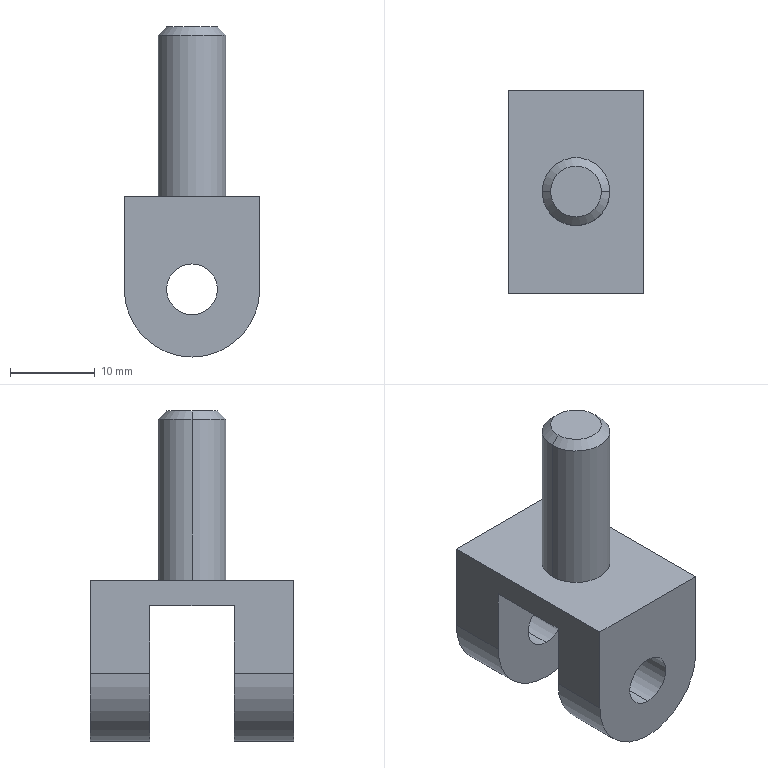Part | SolidWorks | features ICE 3, Chamfer 1, Extrusion 1 | 1 solid | 21 faces | box 16 x 24 x 39 mm | volume 4949 mm3 | cylinder 10 | plane 9 | cone 2 | commonest cylinder face diameters 6 x4 16 x4 8 x2
STEP:
#1=CARTESIAN_POINT('',(3.,0.,31.));
#2=VERTEX_POINT('',#1);
#3=CARTESIAN_POINT('',(-3.,0.,31.));
#4=VERTEX_POINT('',#3);
#5=CARTESIAN_POINT('',(0.,0.,31.));
#6=DIRECTION('',(0.,0.,1.));
#7=DIRECTION('',(1.,0.,0.));
#8=AXIS2_PLACEMENT_3D('',#5,#6,#7);
#9=CIRCLE('',#8,3.);
#10=EDGE_CURVE('',#2,#4,#9,.T.);
#11=ORIENTED_EDGE('',*,*,#10,.F.);
#12=CARTESIAN_POINT('',(4.,0.,30.));
#13=VERTEX_POINT('',#12);
#14=CARTESIAN_POINT('',(3.,0.,31.));
#15=DIRECTION('',(0.7071,0.,-0.7071));
#16=VECTOR('',#15,1000.);
#17=LINE('',#14,#16);
#18=EDGE_CURVE('',#2,#13,#17,.T.);
#19=ORIENTED_EDGE('',*,*,#18,.T.);
#20=CARTESIAN_POINT('',(-4.,0.,30.));
#21=VERTEX_POINT('',#20);
#22=CARTESIAN_POINT('',(0.,0.,30.));
#23=DIRECTION('',(0.,0.,-1.));
#24=DIRECTION('',(1.,0.,0.));
#25=AXIS2_PLACEMENT_3D('',#22,#23,#24);
#26=CIRCLE('',#25,4.);
#27=EDGE_CURVE('',#21,#13,#26,.T.);
#28=ORIENTED_EDGE('',*,*,#27,.F.);
#29=CARTESIAN_POINT('',(-3.,0.,31.));
#30=DIRECTION('',(-0.7071,0.,-0.7071));
#31=VECTOR('',#30,1000.);
#32=LINE('',#29,#31);
#33=EDGE_CURVE('',#4,#21,#32,.T.);
#34=ORIENTED_EDGE('',*,*,#33,.F.);
#35=EDGE_LOOP('',(#11,#19,#28,#34));
#36=FACE_OUTER_BOUND('',#35,.T.);
#37=CARTESIAN_POINT('',(0.,0.,31.));
#38=DIRECTION('',(0.,0.,-1.));
#39=DIRECTION('',(-1.,0.,0.));
#40=AXIS2_PLACEMENT_3D('',#37,#38,#39);
#41=CONICAL_SURFACE('',#40,3.,0.7854);
#42=ADVANCED_FACE('',(#36),#41,.T.);
#43=CARTESIAN_POINT('',(0.,12.,-3.));
#44=VERTEX_POINT('',#43);
#45=CARTESIAN_POINT('',(0.,12.,3.));
#46=VERTEX_POINT('',#45);
#47=CARTESIAN_POINT('',(0.,12.,0.));
#48=DIRECTION('',(0.,1.,0.));
#49=DIRECTION('',(0.,0.,1.));
#50=AXIS2_PLACEMENT_3D('',#47,#48,#49);
#51=CIRCLE('',#50,3.);
#52=EDGE_CURVE('',#44,#46,#51,.T.);
#53=ORIENTED_EDGE('',*,*,#52,.T.);
#54=CARTESIAN_POINT('',(0.,5.,3.));
#55=VERTEX_POINT('',#54);
#56=CARTESIAN_POINT('',(0.,22.,3.));
#57=DIRECTION('',(0.,-1.,0.));
#58=VECTOR('',#57,1000.);
#59=LINE('',#56,#58);
#60=EDGE_CURVE('',#46,#55,#59,.T.);
#61=ORIENTED_EDGE('',*,*,#60,.T.);
#62=CARTESIAN_POINT('',(0.,5.,-3.));
#63=VERTEX_POINT('',#62);
#64=CARTESIAN_POINT('',(0.,5.,0.));
#65=DIRECTION('',(0.,1.,0.));
#66=DIRECTION('',(0.,0.,1.));
#67=AXIS2_PLACEMENT_3D('',#64,#65,#66);
#68=CIRCLE('',#67,3.);
#69=EDGE_CURVE('',#63,#55,#68,.T.);
#70=ORIENTED_EDGE('',*,*,#69,.F.);
#71=CARTESIAN_POINT('',(0.,22.,-3.));
#72=DIRECTION('',(0.,-1.,0.));
#73=VECTOR('',#72,1000.);
#74=LINE('',#71,#73);
#75=EDGE_CURVE('',#44,#63,#74,.T.);
#76=ORIENTED_EDGE('',*,*,#75,.F.);
#77=EDGE_LOOP('',(#53,#61,#70,#76));
#78=FACE_OUTER_BOUND('',#77,.T.);
#79=CARTESIAN_POINT('',(0.,22.,0.));
#80=DIRECTION('',(0.,-1.,0.));
#81=DIRECTION('',(0.,0.,-1.));
#82=AXIS2_PLACEMENT_3D('',#79,#80,#81);
#83=CYLINDRICAL_SURFACE('',#82,3.);
#84=ADVANCED_FACE('',(#78),#83,.F.);
#85=CARTESIAN_POINT('',(0.,-5.,3.));
#86=VERTEX_POINT('',#85);
#87=CARTESIAN_POINT('',(0.,-5.,-3.));
#88=VERTEX_POINT('',#87);
#89=CARTESIAN_POINT('',(0.,-5.,0.));
#90=DIRECTION('',(0.,-1.,0.));
#91=DIRECTION('',(0.,0.,-1.));
#92=AXIS2_PLACEMENT_3D('',#89,#90,#91);
#93=CIRCLE('',#92,3.);
#94=EDGE_CURVE('',#86,#88,#93,.T.);
#95=ORIENTED_EDGE('',*,*,#94,.F.);
#96=CARTESIAN_POINT('',(0.,-12.,3.));
#97=VERTEX_POINT('',#96);
#98=CARTESIAN_POINT('',(0.,22.,3.));
#99=DIRECTION('',(0.,-1.,0.));
#100=VECTOR('',#99,1000.);
#101=LINE('',#98,#100);
#102=EDGE_CURVE('',#86,#97,#101,.T.);
#103=ORIENTED_EDGE('',*,*,#102,.T.);
#104=CARTESIAN_POINT('',(0.,-12.,-3.));
#105=VERTEX_POINT('',#104);
#106=CARTESIAN_POINT('',(0.,-12.,0.));
#107=DIRECTION('',(0.,-1.,0.));
#108=DIRECTION('',(0.,0.,-1.));
#109=AXIS2_PLACEMENT_3D('',#106,#107,#108);
#110=CIRCLE('',#109,3.);
#111=EDGE_CURVE('',#97,#105,#110,.T.);
#112=ORIENTED_EDGE('',*,*,#111,.T.);
#113=CARTESIAN_POINT('',(0.,22.,-3.));
#114=DIRECTION('',(0.,-1.,0.));
#115=VECTOR('',#114,1000.);
#116=LINE('',#113,#115);
#117=EDGE_CURVE('',#88,#105,#116,.T.);
#118=ORIENTED_EDGE('',*,*,#117,.F.);
#119=EDGE_LOOP('',(#95,#103,#112,#118));
#120=FACE_OUTER_BOUND('',#119,.T.);
#121=CARTESIAN_POINT('',(0.,22.,0.));
#122=DIRECTION('',(0.,-1.,0.));
#123=DIRECTION('',(0.,0.,-1.));
#124=AXIS2_PLACEMENT_3D('',#121,#122,#123);
#125=CYLINDRICAL_SURFACE('',#124,3.);
#126=ADVANCED_FACE('',(#120),#125,.F.);
#127=ORIENTED_EDGE('',*,*,#27,.T.);
#128=CARTESIAN_POINT('',(4.,0.,11.));
#129=VERTEX_POINT('',#128);
#130=CARTESIAN_POINT('',(4.,0.,31.));
#131=DIRECTION('',(0.,0.,-1.));
#132=VECTOR('',#131,1000.);
#133=LINE('',#130,#132);
#134=EDGE_CURVE('',#13,#129,#133,.T.);
#135=ORIENTED_EDGE('',*,*,#134,.T.);
#136=CARTESIAN_POINT('',(-4.,0.,11.));
#137=VERTEX_POINT('',#136);
#138=CARTESIAN_POINT('',(0.,0.,11.));
#139=DIRECTION('',(0.,0.,1.));
#140=DIRECTION('',(-1.,0.,0.));
#141=AXIS2_PLACEMENT_3D('',#138,#139,#140);
#142=CIRCLE('',#141,4.);
#143=EDGE_CURVE('',#129,#137,#142,.T.);
#144=ORIENTED_EDGE('',*,*,#143,.T.);
#145=CARTESIAN_POINT('',(-4.,0.,31.));
#146=DIRECTION('',(0.,0.,-1.));
#147=VECTOR('',#146,1000.);
#148=LINE('',#145,#147);
#149=EDGE_CURVE('',#21,#137,#148,.T.);
#150=ORIENTED_EDGE('',*,*,#149,.F.);
#151=EDGE_LOOP('',(#127,#135,#144,#150));
#152=FACE_OUTER_BOUND('',#151,.T.);
#153=CARTESIAN_POINT('',(0.,0.,31.));
#154=DIRECTION('',(0.,0.,-1.));
#155=DIRECTION('',(-1.,0.,0.));
#156=AXIS2_PLACEMENT_3D('',#153,#154,#155);
#157=CYLINDRICAL_SURFACE('',#156,4.);
#158=ADVANCED_FACE('',(#152),#157,.T.);
#159=CARTESIAN_POINT('',(-8.,-5.,0.));
#160=VERTEX_POINT('',#159);
#161=CARTESIAN_POINT('',(0.,-5.,-8.));
#162=VERTEX_POINT('',#161);
#163=CARTESIAN_POINT('',(0.,-5.,0.));
#164=DIRECTION('',(0.,-1.,0.));
#165=DIRECTION('',(0.,0.,-1.));
#166=AXIS2_PLACEMENT_3D('',#163,#164,#165);
#167=CIRCLE('',#166,8.);
#168=EDGE_CURVE('',#160,#162,#167,.T.);
#169=ORIENTED_EDGE('',*,*,#168,.T.);
#170=CARTESIAN_POINT('',(0.,-12.,-8.));
#171=VERTEX_POINT('',#170);
#172=CARTESIAN_POINT('',(0.,12.,-8.));
#173=DIRECTION('',(0.,-1.,0.));
#174=VECTOR('',#173,1000.);
#175=LINE('',#172,#174);
#176=EDGE_CURVE('',#162,#171,#175,.T.);
#177=ORIENTED_EDGE('',*,*,#176,.T.);
#178=CARTESIAN_POINT('',(-8.,-12.,0.));
#179=VERTEX_POINT('',#178);
#180=CARTESIAN_POINT('',(0.,-12.,0.));
#181=DIRECTION('',(0.,1.,0.));
#182=DIRECTION('',(0.,0.,1.));
#183=AXIS2_PLACEMENT_3D('',#180,#181,#182);
#184=CIRCLE('',#183,8.);
#185=EDGE_CURVE('',#171,#179,#184,.T.);
#186=ORIENTED_EDGE('',*,*,#185,.T.);
#187=CARTESIAN_POINT('',(-8.,12.,0.));
#188=DIRECTION('',(0.,-1.,0.));
#189=VECTOR('',#188,1000.);
#190=LINE('',#187,#189);
#191=EDGE_CURVE('',#160,#179,#190,.T.);
#192=ORIENTED_EDGE('',*,*,#191,.F.);
#193=EDGE_LOOP('',(#169,#177,#186,#192));
#194=FACE_OUTER_BOUND('',#193,.T.);
#195=CARTESIAN_POINT('',(0.,12.,0.));
#196=DIRECTION('',(0.,-1.,0.));
#197=DIRECTION('',(0.,0.,-1.));
#198=AXIS2_PLACEMENT_3D('',#195,#196,#197);
#199=CYLINDRICAL_SURFACE('',#198,8.);
#200=ADVANCED_FACE('',(#194),#199,.T.);
#201=CARTESIAN_POINT('',(0.,12.,-8.));
#202=VERTEX_POINT('',#201);
#203=CARTESIAN_POINT('',(-8.,12.,0.));
#204=VERTEX_POINT('',#203);
#205=CARTESIAN_POINT('',(0.,12.,0.));
#206=DIRECTION('',(0.,1.,0.));
#207=DIRECTION('',(0.,0.,1.));
#208=AXIS2_PLACEMENT_3D('',#205,#206,#207);
#209=CIRCLE('',#208,8.);
#210=EDGE_CURVE('',#202,#204,#209,.T.);
#211=ORIENTED_EDGE('',*,*,#210,.F.);
#212=CARTESIAN_POINT('',(0.,5.,-8.));
#213=VERTEX_POINT('',#212);
#214=CARTESIAN_POINT('',(0.,12.,-8.));
#215=DIRECTION('',(0.,-1.,0.));
#216=VECTOR('',#215,1000.);
#217=LINE('',#214,#216);
#218=EDGE_CURVE('',#202,#213,#217,.T.);
#219=ORIENTED_EDGE('',*,*,#218,.T.);
#220=CARTESIAN_POINT('',(-8.,5.,0.));
#221=VERTEX_POINT('',#220);
#222=CARTESIAN_POINT('',(0.,5.,0.));
#223=DIRECTION('',(0.,1.,0.));
#224=DIRECTION('',(0.,0.,1.));
#225=AXIS2_PLACEMENT_3D('',#222,#223,#224);
#226=CIRCLE('',#225,8.);
#227=EDGE_CURVE('',#213,#221,#226,.T.);
#228=ORIENTED_EDGE('',*,*,#227,.T.);
#229=CARTESIAN_POINT('',(-8.,12.,0.));
#230=DIRECTION('',(0.,-1.,0.));
#231=VECTOR('',#230,1000.);
#232=LINE('',#229,#231);
#233=EDGE_CURVE('',#204,#221,#232,.T.);
#234=ORIENTED_EDGE('',*,*,#233,.F.);
#235=EDGE_LOOP('',(#211,#219,#228,#234));
#236=FACE_OUTER_BOUND('',#235,.T.);
#237=CARTESIAN_POINT('',(0.,12.,0.));
#238=DIRECTION('',(0.,-1.,0.));
#239=DIRECTION('',(0.,0.,-1.));
#240=AXIS2_PLACEMENT_3D('',#237,#238,#239);
#241=CYLINDRICAL_SURFACE('',#240,8.);
#242=ADVANCED_FACE('',(#236),#241,.T.);
#243=ORIENTED_EDGE('',*,*,#218,.F.);
#244=CARTESIAN_POINT('',(8.,12.,0.));
#245=VERTEX_POINT('',#244);
#246=CARTESIAN_POINT('',(0.,12.,0.));
#247=DIRECTION('',(0.,1.,0.));
#248=DIRECTION('',(0.,0.,1.));
#249=AXIS2_PLACEMENT_3D('',#246,#247,#248);
#250=CIRCLE('',#249,8.);
#251=EDGE_CURVE('',#245,#202,#250,.T.);
#252=ORIENTED_EDGE('',*,*,#251,.F.);
#253=CARTESIAN_POINT('',(8.,5.,0.));
#254=VERTEX_POINT('',#253);
#255=CARTESIAN_POINT('',(8.,12.,0.));
#256=DIRECTION('',(0.,-1.,0.));
#257=VECTOR('',#256,1000.);
#258=LINE('',#255,#257);
#259=EDGE_CURVE('',#245,#254,#258,.T.);
#260=ORIENTED_EDGE('',*,*,#259,.T.);
#261=CARTESIAN_POINT('',(0.,5.,0.));
#262=DIRECTION('',(0.,1.,0.));
#263=DIRECTION('',(0.,0.,1.));
#264=AXIS2_PLACEMENT_3D('',#261,#262,#263);
#265=CIRCLE('',#264,8.);
#266=EDGE_CURVE('',#254,#213,#265,.T.);
#267=ORIENTED_EDGE('',*,*,#266,.T.);
#268=EDGE_LOOP('',(#243,#252,#260,#267));
#269=FACE_OUTER_BOUND('',#268,.T.);
#270=CARTESIAN_POINT('',(0.,12.,0.));
#271=DIRECTION('',(0.,-1.,0.));
#272=DIRECTION('',(0.,0.,-1.));
#273=AXIS2_PLACEMENT_3D('',#270,#271,#272);
#274=CYLINDRICAL_SURFACE('',#273,8.);
#275=ADVANCED_FACE('',(#269),#274,.T.);
#276=CARTESIAN_POINT('',(-8.,-12.,11.));
#277=VERTEX_POINT('',#276);
#278=CARTESIAN_POINT('',(8.,-12.,11.));
#279=VERTEX_POINT('',#278);
#280=CARTESIAN_POINT('',(-8.,-12.,11.));
#281=DIRECTION('',(1.,0.,0.));
#282=VECTOR('',#281,1000.);
#283=LINE('',#280,#282);
#284=EDGE_CURVE('',#277,#279,#283,.T.);
#285=ORIENTED_EDGE('',*,*,#284,.T.);
#286=CARTESIAN_POINT('',(8.,12.,11.));
#287=VERTEX_POINT('',#286);
#288=CARTESIAN_POINT('',(8.,12.,11.));
#289=DIRECTION('',(0.,-1.,0.));
#290=VECTOR('',#289,1000.);
#291=LINE('',#288,#290);
#292=EDGE_CURVE('',#287,#279,#291,.T.);
#293=ORIENTED_EDGE('',*,*,#292,.F.);
#294=CARTESIAN_POINT('',(-8.,12.,11.));
#295=VERTEX_POINT('',#294);
#296=CARTESIAN_POINT('',(-8.,12.,11.));
#297=DIRECTION('',(1.,0.,0.));
#298=VECTOR('',#297,1000.);
#299=LINE('',#296,#298);
#300=EDGE_CURVE('',#295,#287,#299,.T.);
#301=ORIENTED_EDGE('',*,*,#300,.F.);
#302=CARTESIAN_POINT('',(-8.,12.,11.));
#303=DIRECTION('',(0.,-1.,0.));
#304=VECTOR('',#303,1000.);
#305=LINE('',#302,#304);
#306=EDGE_CURVE('',#295,#277,#305,.T.);
#307=ORIENTED_EDGE('',*,*,#306,.T.);
#308=EDGE_LOOP('',(#285,#293,#301,#307));
#309=FACE_OUTER_BOUND('',#308,.T.);
#310=CARTESIAN_POINT('',(0.,0.,11.));
#311=DIRECTION('',(0.,0.,1.));
#312=DIRECTION('',(-1.,0.,0.));
#313=AXIS2_PLACEMENT_3D('',#310,#311,#312);
#314=CIRCLE('',#313,4.);
#315=EDGE_CURVE('',#137,#129,#314,.T.);
#316=ORIENTED_EDGE('',*,*,#315,.F.);
#317=ORIENTED_EDGE('',*,*,#143,.F.);
#318=EDGE_LOOP('',(#316,#317));
#319=FACE_BOUND('',#318,.T.);
#320=CARTESIAN_POINT('',(-8.,12.,11.));
#321=DIRECTION('',(0.,0.,-1.));
#322=DIRECTION('',(-1.,0.,0.));
#323=AXIS2_PLACEMENT_3D('',#320,#321,#322);
#324=PLANE('',#323);
#325=ADVANCED_FACE('',(#309,#319),#324,.F.);
#326=ORIENTED_EDGE('',*,*,#176,.F.);
#327=CARTESIAN_POINT('',(8.,-5.,0.));
#328=VERTEX_POINT('',#327);
#329=CARTESIAN_POINT('',(0.,-5.,0.));
#330=DIRECTION('',(0.,-1.,0.));
#331=DIRECTION('',(0.,0.,-1.));
#332=AXIS2_PLACEMENT_3D('',#329,#330,#331);
#333=CIRCLE('',#332,8.);
#334=EDGE_CURVE('',#162,#328,#333,.T.);
#335=ORIENTED_EDGE('',*,*,#334,.T.);
#336=CARTESIAN_POINT('',(8.,-12.,0.));
#337=VERTEX_POINT('',#336);
#338=CARTESIAN_POINT('',(8.,12.,0.));
#339=DIRECTION('',(0.,-1.,0.));
#340=VECTOR('',#339,1000.);
#341=LINE('',#338,#340);
#342=EDGE_CURVE('',#328,#337,#341,.T.);
#343=ORIENTED_EDGE('',*,*,#342,.T.);
#344=CARTESIAN_POINT('',(0.,-12.,0.));
#345=DIRECTION('',(0.,1.,0.));
#346=DIRECTION('',(0.,0.,1.));
#347=AXIS2_PLACEMENT_3D('',#344,#345,#346);
#348=CIRCLE('',#347,8.);
#349=EDGE_CURVE('',#337,#171,#348,.T.);
#350=ORIENTED_EDGE('',*,*,#349,.T.);
#351=EDGE_LOOP('',(#326,#335,#343,#350));
#352=FACE_OUTER_BOUND('',#351,.T.);
#353=CARTESIAN_POINT('',(0.,12.,0.));
#354=DIRECTION('',(0.,-1.,0.));
#355=DIRECTION('',(0.,0.,-1.));
#356=AXIS2_PLACEMENT_3D('',#353,#354,#355);
#357=CYLINDRICAL_SURFACE('',#356,8.);
#358=ADVANCED_FACE('',(#352),#357,.T.);
#359=ORIENTED_EDGE('',*,*,#233,.T.);
#360=CARTESIAN_POINT('',(-8.,5.,8.));
#361=VERTEX_POINT('',#360);
#362=CARTESIAN_POINT('',(-8.,5.,0.));
#363=DIRECTION('',(0.,0.,1.));
#364=VECTOR('',#363,1000.);
#365=LINE('',#362,#364);
#366=EDGE_CURVE('',#221,#361,#365,.T.);
#367=ORIENTED_EDGE('',*,*,#366,.T.);
#368=CARTESIAN_POINT('',(-8.,-5.,8.));
#369=VERTEX_POINT('',#368);
#370=CARTESIAN_POINT('',(-8.,12.,8.));
#371=DIRECTION('',(0.,-1.,0.));
#372=VECTOR('',#371,1000.);
#373=LINE('',#370,#372);
#374=EDGE_CURVE('',#361,#369,#373,.T.);
#375=ORIENTED_EDGE('',*,*,#374,.T.);
#376=CARTESIAN_POINT('',(-8.,-5.,0.));
#377=DIRECTION('',(0.,0.,-1.));
#378=VECTOR('',#377,1000.);
#379=LINE('',#376,#378);
#380=EDGE_CURVE('',#369,#160,#379,.T.);
#381=ORIENTED_EDGE('',*,*,#380,.T.);
#382=ORIENTED_EDGE('',*,*,#191,.T.);
#383=CARTESIAN_POINT('',(-8.,-12.,0.));
#384=DIRECTION('',(0.,0.,1.));
#385=VECTOR('',#384,1000.);
#386=LINE('',#383,#385);
#387=EDGE_CURVE('',#179,#277,#386,.T.);
#388=ORIENTED_EDGE('',*,*,#387,.T.);
#389=ORIENTED_EDGE('',*,*,#306,.F.);
#390=CARTESIAN_POINT('',(-8.,12.,0.));
#391=DIRECTION('',(0.,0.,1.));
#392=VECTOR('',#391,1000.);
#393=LINE('',#390,#392);
#394=EDGE_CURVE('',#204,#295,#393,.T.);
#395=ORIENTED_EDGE('',*,*,#394,.F.);
#396=EDGE_LOOP('',(#359,#367,#375,#381,#382,#388,#389,#395));
#397=FACE_OUTER_BOUND('',#396,.T.);
#398=CARTESIAN_POINT('',(-8.,12.,0.));
#399=DIRECTION('',(1.,0.,0.));
#400=DIRECTION('',(0.,0.,-1.));
#401=AXIS2_PLACEMENT_3D('',#398,#399,#400);
#402=PLANE('',#401);
#403=ADVANCED_FACE('',(#397),#402,.F.);
#404=CARTESIAN_POINT('',(8.,5.,8.));
#405=VERTEX_POINT('',#404);
#406=CARTESIAN_POINT('',(8.,-5.,8.));
#407=VERTEX_POINT('',#406);
#408=CARTESIAN_POINT('',(8.,5.,8.));
#409=DIRECTION('',(0.,-1.,0.));
#410=VECTOR('',#409,1000.);
#411=LINE('',#408,#410);
#412=EDGE_CURVE('',#405,#407,#411,.T.);
#413=ORIENTED_EDGE('',*,*,#412,.F.);
#414=CARTESIAN_POINT('',(8.,5.,0.));
#415=DIRECTION('',(0.,0.,-1.));
#416=VECTOR('',#415,1000.);
#417=LINE('',#414,#416);
#418=EDGE_CURVE('',#405,#254,#417,.T.);
#419=ORIENTED_EDGE('',*,*,#418,.T.);
#420=ORIENTED_EDGE('',*,*,#259,.F.);
#421=CARTESIAN_POINT('',(8.,12.,0.));
#422=DIRECTION('',(0.,0.,-1.));
#423=VECTOR('',#422,1000.);
#424=LINE('',#421,#423);
#425=EDGE_CURVE('',#287,#245,#424,.T.);
#426=ORIENTED_EDGE('',*,*,#425,.F.);
#427=ORIENTED_EDGE('',*,*,#292,.T.);
#428=CARTESIAN_POINT('',(8.,-12.,0.));
#429=DIRECTION('',(0.,0.,-1.));
#430=VECTOR('',#429,1000.);
#431=LINE('',#428,#430);
#432=EDGE_CURVE('',#279,#337,#431,.T.);
#433=ORIENTED_EDGE('',*,*,#432,.T.);
#434=ORIENTED_EDGE('',*,*,#342,.F.);
#435=CARTESIAN_POINT('',(8.,-5.,-24.));
#436=DIRECTION('',(0.,0.,-1.));
#437=VECTOR('',#436,1000.);
#438=LINE('',#435,#437);
#439=EDGE_CURVE('',#407,#328,#438,.T.);
#440=ORIENTED_EDGE('',*,*,#439,.F.);
#441=EDGE_LOOP('',(#413,#419,#420,#426,#427,#433,#434,#440));
#442=FACE_OUTER_BOUND('',#441,.T.);
#443=CARTESIAN_POINT('',(8.,12.,0.));
#444=DIRECTION('',(-1.,0.,0.));
#445=DIRECTION('',(0.,0.,1.));
#446=AXIS2_PLACEMENT_3D('',#443,#444,#445);
#447=PLANE('',#446);
#448=ADVANCED_FACE('',(#442),#447,.F.);
#449=ORIENTED_EDGE('',*,*,#52,.F.);
#450=CARTESIAN_POINT('',(0.,12.,0.));
#451=DIRECTION('',(0.,1.,0.));
#452=DIRECTION('',(0.,0.,1.));
#453=AXIS2_PLACEMENT_3D('',#450,#451,#452);
#454=CIRCLE('',#453,3.);
#455=EDGE_CURVE('',#46,#44,#454,.T.);
#456=ORIENTED_EDGE('',*,*,#455,.F.);
#457=EDGE_LOOP('',(#449,#456));
#458=FACE_BOUND('',#457,.T.);
#459=ORIENTED_EDGE('',*,*,#251,.T.);
#460=ORIENTED_EDGE('',*,*,#210,.T.);
#461=ORIENTED_EDGE('',*,*,#394,.T.);
#462=ORIENTED_EDGE('',*,*,#300,.T.);
#463=ORIENTED_EDGE('',*,*,#425,.T.);
#464=EDGE_LOOP('',(#459,#460,#461,#462,#463));
#465=FACE_OUTER_BOUND('',#464,.T.);
#466=CARTESIAN_POINT('',(0.,12.,0.));
#467=DIRECTION('',(0.,1.,0.));
#468=DIRECTION('',(0.,0.,1.));
#469=AXIS2_PLACEMENT_3D('',#466,#467,#468);
#470=PLANE('',#469);
#471=ADVANCED_FACE('',(#458,#465),#470,.T.);
#472=CARTESIAN_POINT('',(0.,-12.,0.));
#473=DIRECTION('',(0.,-1.,0.));
#474=DIRECTION('',(0.,0.,-1.));
#475=AXIS2_PLACEMENT_3D('',#472,#473,#474);
#476=CIRCLE('',#475,3.);
#477=EDGE_CURVE('',#105,#97,#476,.T.);
#478=ORIENTED_EDGE('',*,*,#477,.F.);
#479=ORIENTED_EDGE('',*,*,#111,.F.);
#480=EDGE_LOOP('',(#478,#479));
#481=FACE_BOUND('',#480,.T.);
#482=ORIENTED_EDGE('',*,*,#349,.F.);
#483=ORIENTED_EDGE('',*,*,#432,.F.);
#484=ORIENTED_EDGE('',*,*,#284,.F.);
#485=ORIENTED_EDGE('',*,*,#387,.F.);
#486=ORIENTED_EDGE('',*,*,#185,.F.);
#487=EDGE_LOOP('',(#482,#483,#484,#485,#486));
#488=FACE_OUTER_BOUND('',#487,.T.);
#489=CARTESIAN_POINT('',(0.,-12.,0.));
#490=DIRECTION('',(0.,1.,0.));
#491=DIRECTION('',(0.,0.,1.));
#492=AXIS2_PLACEMENT_3D('',#489,#490,#491);
#493=PLANE('',#492);
#494=ADVANCED_FACE('',(#481,#488),#493,.F.);
#495=ORIENTED_EDGE('',*,*,#134,.F.);
#496=CARTESIAN_POINT('',(0.,0.,30.));
#497=DIRECTION('',(0.,0.,-1.));
#498=DIRECTION('',(1.,0.,0.));
#499=AXIS2_PLACEMENT_3D('',#496,#497,#498);
#500=CIRCLE('',#499,4.);
#501=EDGE_CURVE('',#13,#21,#500,.T.);
#502=ORIENTED_EDGE('',*,*,#501,.T.);
#503=ORIENTED_EDGE('',*,*,#149,.T.);
#504=ORIENTED_EDGE('',*,*,#315,.T.);
#505=EDGE_LOOP('',(#495,#502,#503,#504));
#506=FACE_OUTER_BOUND('',#505,.T.);
#507=CARTESIAN_POINT('',(0.,0.,31.));
#508=DIRECTION('',(0.,0.,-1.));
#509=DIRECTION('',(-1.,0.,0.));
#510=AXIS2_PLACEMENT_3D('',#507,#508,#509);
#511=CYLINDRICAL_SURFACE('',#510,4.);
#512=ADVANCED_FACE('',(#506),#511,.T.);
#513=CARTESIAN_POINT('',(0.,0.,31.));
#514=DIRECTION('',(0.,0.,1.));
#515=DIRECTION('',(1.,0.,0.));
#516=AXIS2_PLACEMENT_3D('',#513,#514,#515);
#517=CIRCLE('',#516,3.);
#518=EDGE_CURVE('',#4,#2,#517,.T.);
#519=ORIENTED_EDGE('',*,*,#518,.T.);
#520=ORIENTED_EDGE('',*,*,#10,.T.);
#521=EDGE_LOOP('',(#519,#520));
#522=FACE_OUTER_BOUND('',#521,.T.);
#523=CARTESIAN_POINT('',(0.,0.,31.));
#524=DIRECTION('',(0.,0.,1.));
#525=DIRECTION('',(1.,0.,0.));
#526=AXIS2_PLACEMENT_3D('',#523,#524,#525);
#527=PLANE('',#526);
#528=ADVANCED_FACE('',(#522),#527,.T.);
#529=CARTESIAN_POINT('',(-12.,5.,8.));
#530=DIRECTION('',(1.,0.,0.));
#531=VECTOR('',#530,1000.);
#532=LINE('',#529,#531);
#533=EDGE_CURVE('',#361,#405,#532,.T.);
#534=ORIENTED_EDGE('',*,*,#533,.T.);
#535=ORIENTED_EDGE('',*,*,#412,.T.);
#536=CARTESIAN_POINT('',(-12.,-5.,8.));
#537=DIRECTION('',(1.,0.,0.));
#538=VECTOR('',#537,1000.);
#539=LINE('',#536,#538);
#540=EDGE_CURVE('',#369,#407,#539,.T.);
#541=ORIENTED_EDGE('',*,*,#540,.F.);
#542=ORIENTED_EDGE('',*,*,#374,.F.);
#543=EDGE_LOOP('',(#534,#535,#541,#542));
#544=FACE_OUTER_BOUND('',#543,.T.);
#545=CARTESIAN_POINT('',(-12.,5.,8.));
#546=DIRECTION('',(0.,0.,1.));
#547=DIRECTION('',(1.,0.,0.));
#548=AXIS2_PLACEMENT_3D('',#545,#546,#547);
#549=PLANE('',#548);
#550=ADVANCED_FACE('',(#544),#549,.F.);
#551=ORIENTED_EDGE('',*,*,#69,.T.);
#552=CARTESIAN_POINT('',(0.,5.,0.));
#553=DIRECTION('',(0.,1.,0.));
#554=DIRECTION('',(0.,0.,1.));
#555=AXIS2_PLACEMENT_3D('',#552,#553,#554);
#556=CIRCLE('',#555,3.);
#557=EDGE_CURVE('',#55,#63,#556,.T.);
#558=ORIENTED_EDGE('',*,*,#557,.T.);
#559=EDGE_LOOP('',(#551,#558));
#560=FACE_BOUND('',#559,.T.);
#561=ORIENTED_EDGE('',*,*,#418,.F.);
#562=ORIENTED_EDGE('',*,*,#533,.F.);
#563=ORIENTED_EDGE('',*,*,#366,.F.);
#564=ORIENTED_EDGE('',*,*,#227,.F.);
#565=ORIENTED_EDGE('',*,*,#266,.F.);
#566=EDGE_LOOP('',(#561,#562,#563,#564,#565));
#567=FACE_OUTER_BOUND('',#566,.T.);
#568=CARTESIAN_POINT('',(-12.,5.,-24.));
#569=DIRECTION('',(0.,1.,0.));
#570=DIRECTION('',(0.,0.,1.));
#571=AXIS2_PLACEMENT_3D('',#568,#569,#570);
#572=PLANE('',#571);
#573=ADVANCED_FACE('',(#560,#567),#572,.F.);
#574=CARTESIAN_POINT('',(0.,-5.,0.));
#575=DIRECTION('',(0.,-1.,0.));
#576=DIRECTION('',(0.,0.,-1.));
#577=AXIS2_PLACEMENT_3D('',#574,#575,#576);
#578=CIRCLE('',#577,3.);
#579=EDGE_CURVE('',#88,#86,#578,.T.);
#580=ORIENTED_EDGE('',*,*,#579,.T.);
#581=ORIENTED_EDGE('',*,*,#94,.T.);
#582=EDGE_LOOP('',(#580,#581));
#583=FACE_BOUND('',#582,.T.);
#584=ORIENTED_EDGE('',*,*,#380,.F.);
#585=ORIENTED_EDGE('',*,*,#540,.T.);
#586=ORIENTED_EDGE('',*,*,#439,.T.);
#587=ORIENTED_EDGE('',*,*,#334,.F.);
#588=ORIENTED_EDGE('',*,*,#168,.F.);
#589=EDGE_LOOP('',(#584,#585,#586,#587,#588));
#590=FACE_OUTER_BOUND('',#589,.T.);
#591=CARTESIAN_POINT('',(-12.,-5.,-24.));
#592=DIRECTION('',(0.,-1.,0.));
#593=DIRECTION('',(0.,0.,-1.));
#594=AXIS2_PLACEMENT_3D('',#591,#592,#593);
#595=PLANE('',#594);
#596=ADVANCED_FACE('',(#583,#590),#595,.F.);
#597=ORIENTED_EDGE('',*,*,#102,.F.);
#598=ORIENTED_EDGE('',*,*,#579,.F.);
#599=ORIENTED_EDGE('',*,*,#117,.T.);
#600=ORIENTED_EDGE('',*,*,#477,.T.);
#601=EDGE_LOOP('',(#597,#598,#599,#600));
#602=FACE_OUTER_BOUND('',#601,.T.);
#603=CARTESIAN_POINT('',(0.,22.,0.));
#604=DIRECTION('',(0.,-1.,0.));
#605=DIRECTION('',(0.,0.,-1.));
#606=AXIS2_PLACEMENT_3D('',#603,#604,#605);
#607=CYLINDRICAL_SURFACE('',#606,3.);
#608=ADVANCED_FACE('',(#602),#607,.F.);
#609=ORIENTED_EDGE('',*,*,#60,.F.);
#610=ORIENTED_EDGE('',*,*,#455,.T.);
#611=ORIENTED_EDGE('',*,*,#75,.T.);
#612=ORIENTED_EDGE('',*,*,#557,.F.);
#613=EDGE_LOOP('',(#609,#610,#611,#612));
#614=FACE_OUTER_BOUND('',#613,.T.);
#615=CARTESIAN_POINT('',(0.,22.,0.));
#616=DIRECTION('',(0.,-1.,0.));
#617=DIRECTION('',(0.,0.,-1.));
#618=AXIS2_PLACEMENT_3D('',#615,#616,#617);
#619=CYLINDRICAL_SURFACE('',#618,3.);
#620=ADVANCED_FACE('',(#614),#619,.F.);
#621=ORIENTED_EDGE('',*,*,#18,.F.);
#622=ORIENTED_EDGE('',*,*,#518,.F.);
#623=ORIENTED_EDGE('',*,*,#33,.T.);
#624=ORIENTED_EDGE('',*,*,#501,.F.);
#625=EDGE_LOOP('',(#621,#622,#623,#624));
#626=FACE_OUTER_BOUND('',#625,.T.);
#627=CARTESIAN_POINT('',(0.,0.,31.));
#628=DIRECTION('',(0.,0.,-1.));
#629=DIRECTION('',(-1.,0.,0.));
#630=AXIS2_PLACEMENT_3D('',#627,#628,#629);
#631=CONICAL_SURFACE('',#630,3.,0.7854);
#632=ADVANCED_FACE('',(#626),#631,.T.);
#633=CLOSED_SHELL('',(#42,#84,#126,#158,#200,#242,#275,#325,#358,#403,#448,#471,#494,#512,#528,#550,#573,#596,#608,#620,#632));
#634=MANIFOLD_SOLID_BREP('',#633);
#635=CARTESIAN_POINT('',(0.,0.,0.));
#636=DIRECTION('',(0.,0.,1.));
#637=DIRECTION('',(1.,0.,0.));
#638=AXIS2_PLACEMENT_3D('',#635,#636,#637);
#639=(LENGTH_UNIT()NAMED_UNIT(*)SI_UNIT(.MILLI.,.METRE.));
#640=UNCERTAINTY_MEASURE_WITH_UNIT(LENGTH_MEASURE(0.00001),#639,'','');
#641=(NAMED_UNIT(*)PLANE_ANGLE_UNIT()SI_UNIT($,.RADIAN.));
#642=(NAMED_UNIT(*)SI_UNIT($,.STERADIAN.)SOLID_ANGLE_UNIT());
#643=(GEOMETRIC_REPRESENTATION_CONTEXT(3)GLOBAL_UNCERTAINTY_ASSIGNED_CONTEXT((#640))GLOBAL_UNIT_ASSIGNED_CONTEXT((#639,#641,#642))REPRESENTATION_CONTEXT('',''));
#644=ADVANCED_BREP_SHAPE_REPRESENTATION('',(#634,#638),#643);